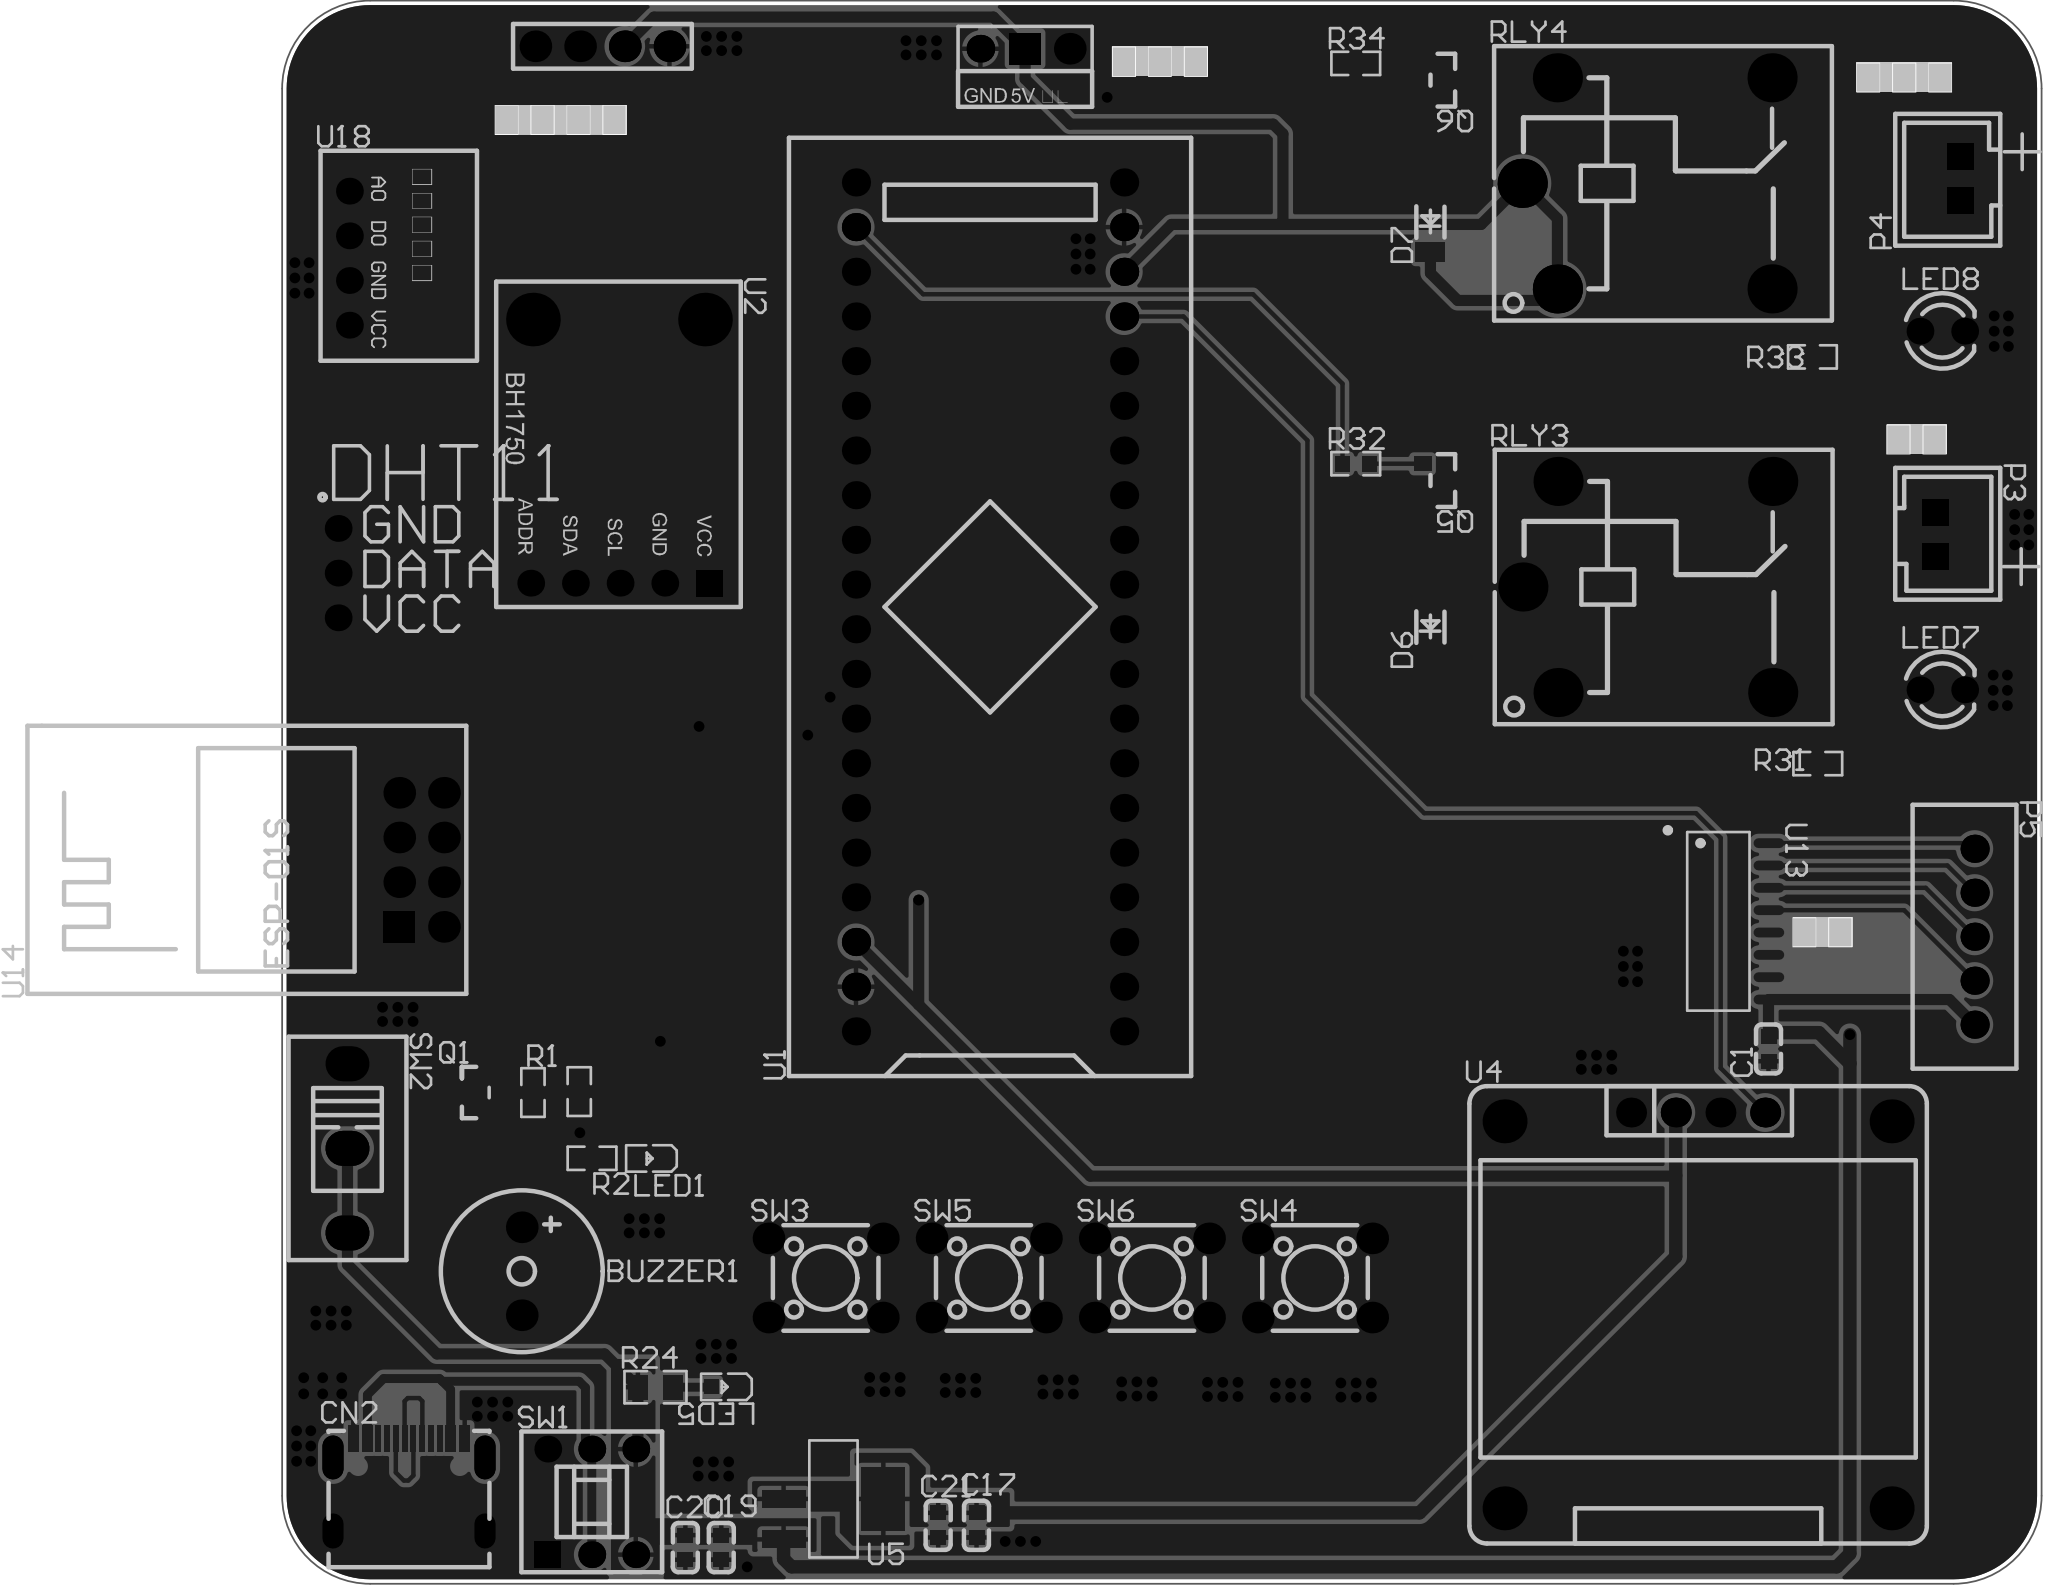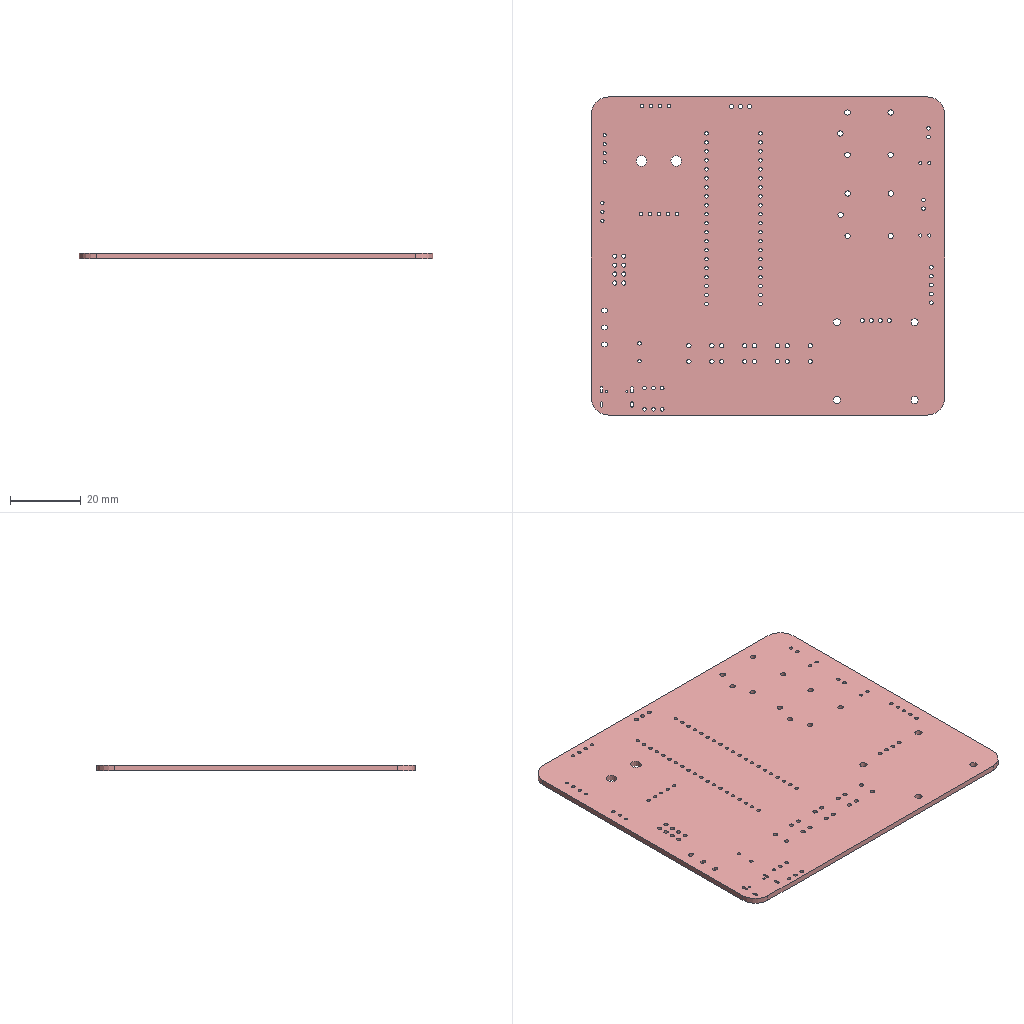Circuit board layout | Altium Designer | box 100 x 90 x 1.6 mm
Layer stack:
# Altium Designer layer stack of  (unit mm; dielectric type: 0 none, 1 core, 2 prepreg, 3 surface material)
index,name,kind,layer,copper_thickness_mm,dielectric_type,dielectric_thickness_mm,dielectric_material,dielectric_constant
0,Top Paste Mask Layer,other,,,,,,
1,Top Silkscreen Layer,other,,,,,,
2,Top Solder Mask Layer,dielectric,,,3,0.01,,3.3
3,Top Layer,copper,Top Layer,0.035,,,,
4,Dielectric1,dielectric,,,3,1.51,FR4,4.5
5,Bottom Layer,copper,Bottom Layer,0.035,,,,
6,Bottom Solder Mask Layer,dielectric,,,3,0.01,,3.3
7,Bottom Silkscreen Layer,other,,,,,,
8,Bottom Paste Mask Layer,other,,,,,,
# drill layer pairs: low layer,high layer
drill_pair,Top Layer,Bottom Layer
Part placement:
Designator,Comment,Layer,Footprint,Center-X(mm),Center-Y(mm),Rotation
CN2,USB-TYPEC,TopLayer,USB-C-SMD_MC-307,100.742,85.688,0
R28,1k,TopLayer,R0603,110.417,108.025,270
R24,4.7k,TopLayer,R0805,114.75,91.221,0
C20,10u,TopLayer,C0603,116.45,82.112,90
LED5,,TopLayer,LED_0603,118.734,91.246,180
C19,100n,TopLayer,C0603,118.492,82.112,90
U5,TLV1117LV33DCYT,TopLayer,SOT-223-4_L6.5-W3.5-P2.30-LS7.0-BR,124.866,84.87,180
C21,22u,TopLayer,C0603,130.821,83.379,90
C17,100n,TopLayer,C0603,132.998,83.379,90
R34,1k,TopLayer,R0603,154.552,166.475,0
R32,1k,TopLayer,R0603,154.552,143.72,0
Q6,,TopLayer,S8050_SOT-23,159.5,165.524,180
Q5,,TopLayer,S8050_SOT-23,159.5,142.762,180
D7,LL4148,TopLayer,LL-34_L3.5-W1.5-RD,158.795,157.454,90
D6,LL4148,TopLayer,LL-34_L3.5-W1.5-RD,158.795,134.431,90
U13,ULN2003A,TopLayer,SOP-16_L10.0-W3.9-P1.27-LS6.0-BL,175.161,117.704,270
C1,47pf,TopLayer,C0603,178.01,110.451,90
R33,3.3k,TopLayer,R0603,180.508,149.791,0
R31,3.3k,TopLayer,R0603,180.812,126.671,0
U20,,TopLayer,dht11温湿度传感器,96.715,137.5,0
U18,光照强度模块,TopLayer,光敏传感器,97.355,155.403,0
U14,ESP-01S,TopLayer,WIFIM-TH_ESP-01S,101.459,121.201,90
BUZZER1,HNB09A03,TopLayer,BUZ-TH_BD9.0-P5.00-D0.6-FD,107.152,97.812,270
U19,,TopLayer,4P排母,111.736,167.448,180
SW1,K8-8081D-NNW,TopLayer,SW-TH_6P-L8.0-W8.0-P2.50,111.13,84.703,0
U1,LCKFB-DKX-STM32F103C8T6,TopLayer,CONN-TH_L53.3-W22.9_STM32F103C8T6-CARD,133.767,135.579,90
H1,舵机模块,TopLayer,舵机模块,135.758,167.309,0
U4,,TopLayer,OLED_I2C_0.96,174.01,95.586,0
RLY4,SRD-05VDC-SL-C,TopLayer,RELAY-TH_SRD-XXVDC-XL-C,171.113,159.658,0
RLY3,SRD-05VDC-SL-C,TopLayer,RELAY-TH_SRD-XXVDC-XL-C,171.151,136.712,0
LED8,,TopLayer,LED_TH-3mm,187.89,151.253,0
LED7,,TopLayer,LED_TH-3mm,187.89,130.867,0
P3,XH2.54直插座-2P,TopLayer,CONN-TH_XH2.54-2P,187.5,139.674,270
P4,XH2.54直插座-2P,TopLayer,CONN-TH_XH2.54-2P,188.897,159.924,90
P5,,TopLayer,CONN-TH_XH2.54-5P,189.726,116.831,270
U2,,TopLayer,BH1750光照传感器,112.739,144.421,270
LED1,,TopLayer,LED_0603,114.471,104.231,180
Q1,,TopLayer,S8550P_SOT,104.399,107.972,0
R1,10k,TopLayer,R0603,107.786,107.972,270
R2,1k,TopLayer,R0603,111.144,104.233,180
SW3,,TopLayer,SW-TH_4P-L6.0-W6.0-P4.50-LS6.5,124.423,97.431,0
SW4,,TopLayer,SW-TH_4P-L6.0-W6.0-P4.50-LS6.5,152.236,97.431,0
SW5,,TopLayer,SW-TH_4P-L6.0-W6.0-P4.50-LS6.5,133.694,97.431,0
SW6,,TopLayer,SW-TH_4P-L6.0-W6.0-P4.50-LS6.5,142.965,97.431,0
SW2,XY-SS12D10L3,TopLayer,SW-TH_3P-L12.7-W6.7_XY-SS12D10LXX,97.245,104.797,270
Pad and via stacks:
# Altium Designer via and pad stacks of  (unit mm). Each distinct definition once, with the count of objects using it.
# via: kind,start_layer,end_layer,hole_mm,diameter_mm,mode(0 simple;1 top-mid-bottom;2 full stack),diameter_per_layer,count,example_net
# pad: kind,layer,hole_mm,hole_type(0 round;1 square;2 slot),plating,top_size,top_shape(1 round;2 rect;3 octagon;9 rounded rect),mid_size,bottom_size,mode,footprint,size_per_layer,count,example
pad,Top Layer,0,0,plated,0.6x1.524,2,0.6x1.524,0.6x1.524,0,USB-C-SMD_MC-307,,4,CN2.A1B12
pad,Top Layer,0,0,plated,0.3x1.524,2,0.3x1.524,0.3x1.524,0,USB-C-SMD_MC-307,,8,CN2.B5
pad,Top Layer,0,0,plated,0.8065x0.864,2,0.8065x0.864,0.8065x0.864,0,R0603,,14,R28.2
pad,Top Layer,0,0,plated,1.133x1.377,2,1.133x1.377,1.133x1.377,0,R0805,,2,R24.2
pad,Top Layer,0,0,plated,0.8x0.9,2,0.8x0.9,0.8x0.9,0,C0603,,10,C20.2
pad,Top Layer,0,0,plated,0.8001x0.8001,2,0.8001x0.8001,0.8001x0.8001,0,LED_0603,,4,LED5.1
pad,Top Layer,0,0,plated,2.47x0.98,2,2.47x0.98,2.47x0.98,0,SOT-223-4_L6.5-W3.5-P2.30-LS7.0-BR,,3,U5.1
pad,Top Layer,0,0,plated,2.47x3.6,2,2.47x3.6,2.47x3.6,0,SOT-223-4_L6.5-W3.5-P2.30-LS7.0-BR,,1,U5.4
pad,Top Layer,0,0,plated,1x0.8,2,1x0.8,1x0.8,0,S8050_SOT-23,,6,Q6.2
pad,Top Layer,0,0,plated,1.1x1.7,2,1.1x1.7,1.1x1.7,0,LL-34_L3.5-W1.5-RD,,4,D7.2
pad,Top Layer,0,0,plated,0.56x1.745,1,0.56x1.745,0.56x1.745,0,SOP-16_L10.0-W3.9-P1.27-LS6.0-BL,,16,U13.1
pad,Top Layer,0,0,plated,0.701x1.25,2,0.701x1.25,0.701x1.25,0,S8550P_SOT,,3,Q1.3
pad,Multi-Layer,0.7,2,plated,1.2x2,1,1.2x2,1.2x2,0,USB-C-SMD_MC-307,,2,CN2.0
pad,Multi-Layer,0.7,2,plated,1.2x2.5,1,1.2x2.5,1.2x2.5,0,USB-C-SMD_MC-307,,2,CN2.2
pad,Multi-Layer,0.9144,0,plated,1.524x1.524,1,1.524x1.524,1.524x1.524,0,dht11\u00CE\u00C2\u00CA\u00AA\u00B6\u00C8\u00B4\u00AB\u00B8\u00D0\u00C6\u00F7,,3,U20.1
pad,Multi-Layer,0.9144,2,plated,1.524x1.524,1,1.524x1.524,1.524x1.524,0,\u00B9\u00E2\u00C3\u00F4\u00B4\u00AB\u00B8\u00D0\u00C6\u00F7,,4,U18.1
pad,Multi-Layer,1.2,0,plated,1.8x1.8,2,1.8x1.8,1.8x1.8,0,WIFIM-TH_ESP-01S,,1,U14.1
pad,Multi-Layer,1.2,0,plated,1.8x1.8,1,1.8x1.8,1.8x1.8,0,WIFIM-TH_ESP-01S,,7,U14.2
pad,Multi-Layer,1,0,plated,1.8x1.8,1,1.8x1.8,1.8x1.8,0,BUZ-TH_BD9.0-P5.00-D0.6-FD,,2,BUZZER1.1
pad,Multi-Layer,1,0,plated,1.8x1.8,1,1.8x1.8,1.8x1.8,0,4P\u00C5\u00C5\u00C4\u00B8,,4,U19.1
pad,Multi-Layer,1,0,plated,1.524x1.524,1,1.524x1.524,1.524x1.524,0,SW-TH_6P-L8.0-W8.0-P2.50,,5,SW1.3
pad,Multi-Layer,1,0,plated,1.524x1.524,2,1.524x1.524,1.524x1.524,0,SW-TH_6P-L8.0-W8.0-P2.50,,1,SW1.1
pad,Multi-Layer,1,0,plated,1.6x1.6,1,1.6x1.6,1.6x1.6,0,CONN-TH_L53.3-W22.9_STM32F103C8T6-CARD,,40,U1.1
pad,Multi-Layer,1.2,0,plated,1.8x1.8,1,1.8x1.8,1.8x1.8,0,\u00B6\u00E6\u00BB\u00FA\u00C4\u00A3\u00BF\u00E9,,1,H1.3
pad,Multi-Layer,1.2,0,plated,1.8x1.8,2,1.8x1.8,1.8x1.8,0,\u00B6\u00E6\u00BB\u00FA\u00C4\u00A3\u00BF\u00E9,,1,H1.2
pad,Multi-Layer,1.2,0,plated,1.575x1.575,1,1.575x1.575,1.575x1.575,0,\u00B6\u00E6\u00BB\u00FA\u00C4\u00A3\u00BF\u00E9,,1,H1.1
pad,Multi-Layer,1.1,0,plated,1.7x1.7,1,1.7x1.7,1.7x1.7,0,OLED_I2C_0.96,,4,U4.1
pad,Multi-Layer,2,0,plated,2.5x2.5,1,2.5x2.5,2.5x2.5,0,OLED_I2C_0.96,,4,U4.5
pad,Multi-Layer,1.524,0,plated,2.794x2.794,1,2.794x2.794,2.794x2.794,0,RELAY-TH_SRD-XXVDC-XL-C,,10,RLY4.2
pad,Multi-Layer,0.9144,0,plated,1.524x1.524,1,1.524x1.524,1.524x1.524,0,LED_TH-3mm,,4,LED8.1
pad,Multi-Layer,1,2,plated,1.524x1.524,2,1.524x1.524,1.524x1.524,0,CONN-TH_XH2.54-2P,,4,P3.1
pad,Multi-Layer,1,0,plated,1.6x1.6,1,1.6x1.6,1.6x1.6,0,CONN-TH_XH2.54-5P,,5,P5.1
pad,Multi-Layer,3.048,0,unplated,3.048x3.048,1,3.048x3.048,3.048x3.048,0,BH1750\u00B9\u00E2\u00D5\u00D5\u00B4\u00AB\u00B8\u00D0\u00C6\u00F7,,2,U2.
pad,Multi-Layer,0.9144,0,plated,1.524x1.524,2,1.524x1.524,1.524x1.524,0,BH1750\u00B9\u00E2\u00D5\u00D5\u00B4\u00AB\u00B8\u00D0\u00C6\u00F7,,1,U2.1
pad,Multi-Layer,0.9144,0,plated,1.524x1.524,1,1.524x1.524,1.524x1.524,0,BH1750\u00B9\u00E2\u00D5\u00D5\u00B4\u00AB\u00B8\u00D0\u00C6\u00F7,,4,U2.4
pad,Multi-Layer,1.2,0,plated,1.8x1.8,1,1.8x1.8,1.8x1.8,0,SW-TH_4P-L6.0-W6.0-P4.50-LS6.5,,16,SW3.1
pad,Multi-Layer,1.2,2,plated,2x2.5,1,2x2.5,2x2.5,0,SW-TH_3P-L12.7-W6.7_XY-SS12D10LXX,,3,SW2.1
via,Top Layer,Bottom Layer,0.3048,0.61,0,,156,GND
Copper pours:
name,layer,net,type(0 solid;1 hatched;2 none)
Bottom Layer-GND,Bottom Layer,GND,0
Top Layer-+5V,Top Layer,+5V,0
Top Layer-VCC,Top Layer,VCC,0
Top Layer-GND,Top Layer,GND,0